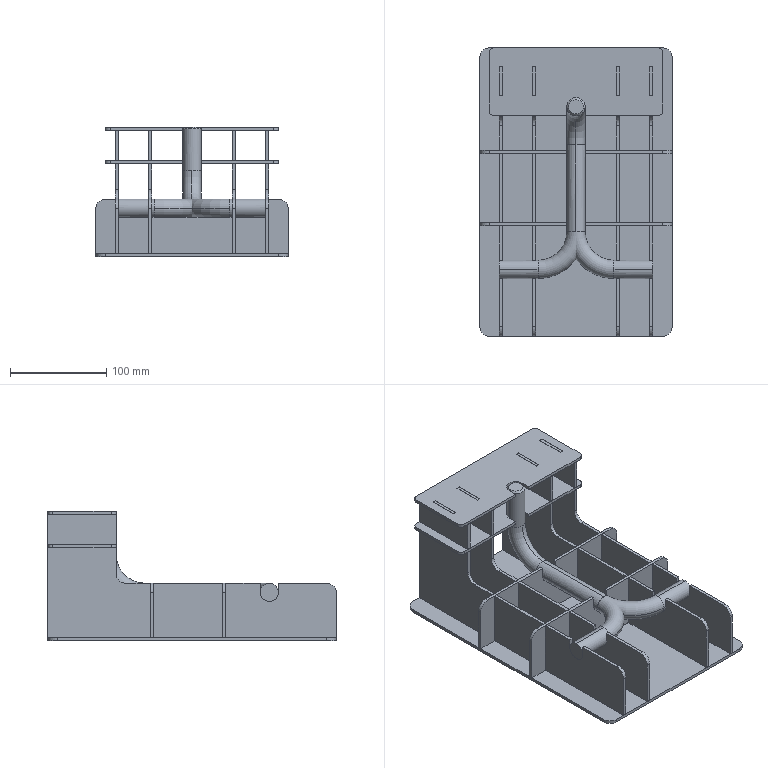Part | SolidWorks | features ReferencePattern 4, LocalLPattern 3, MirrorCompFeat 1 | 11 solids | 386 faces | box 200 x 300 x 135 mm | volume 782542 mm3 | plane 330 | cylinder 44 | torus 8 | cone 4 | commonest cylinder face diameters 19 x20 20 x16 10 x8